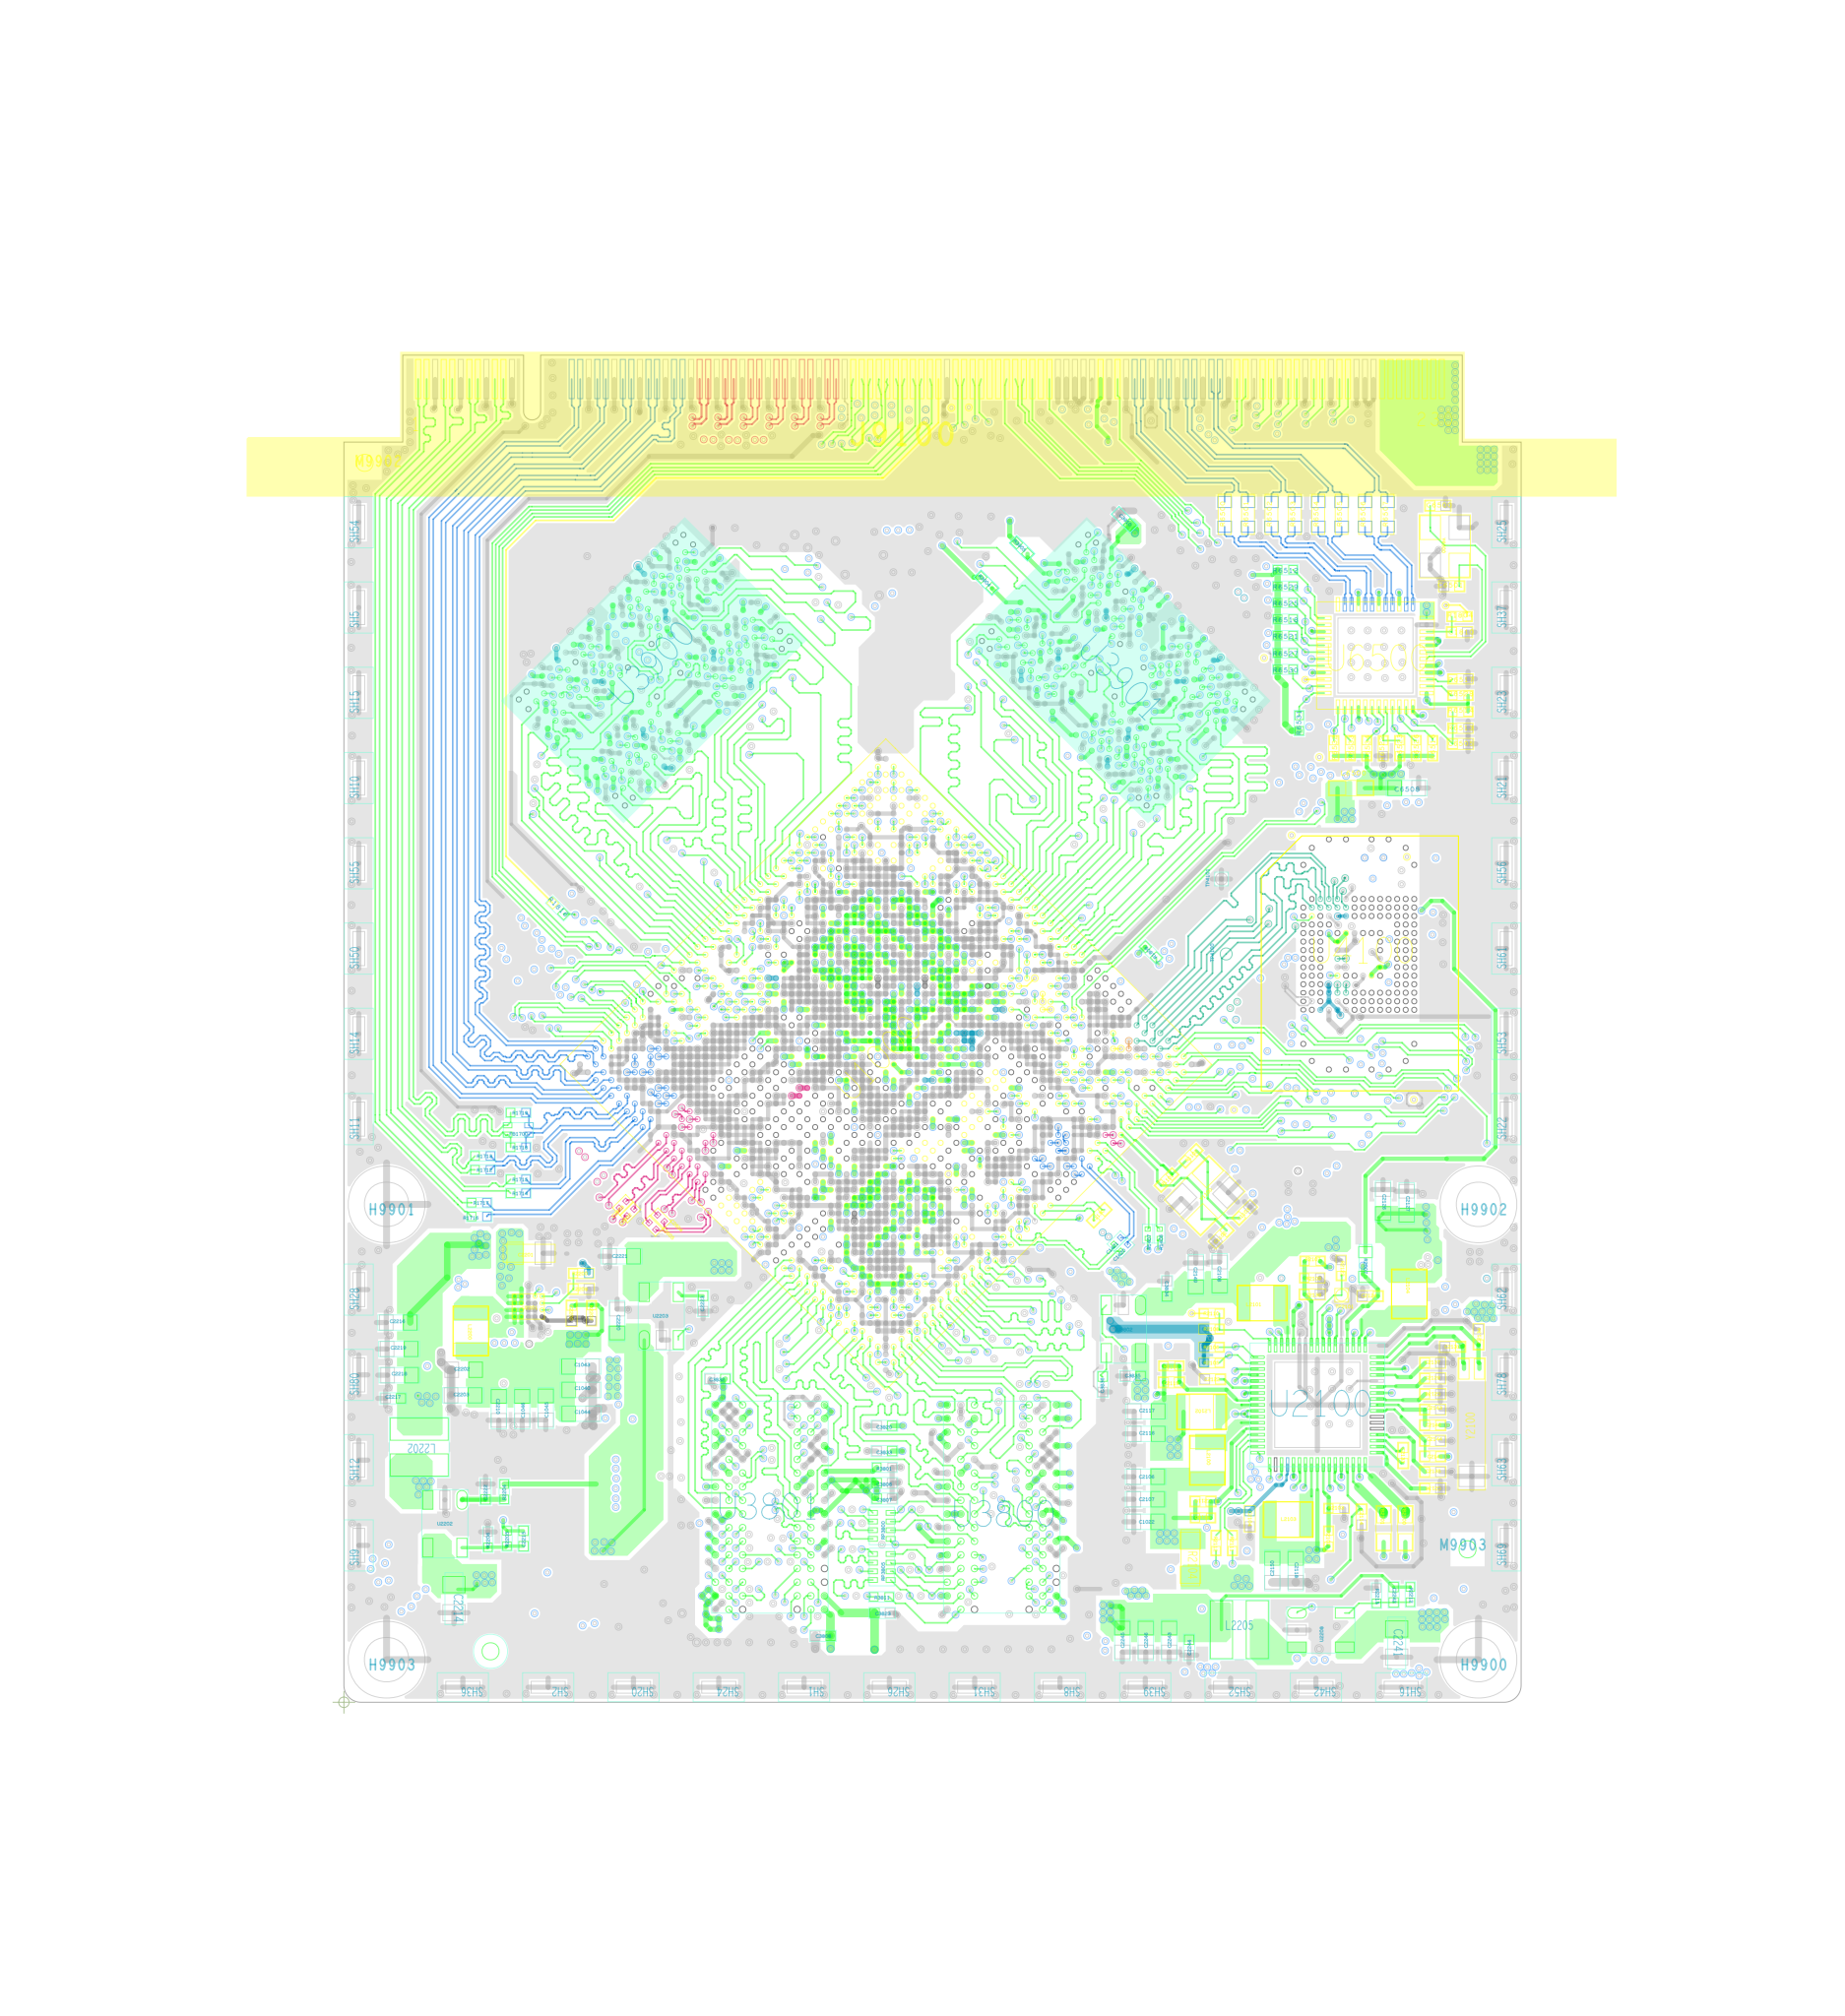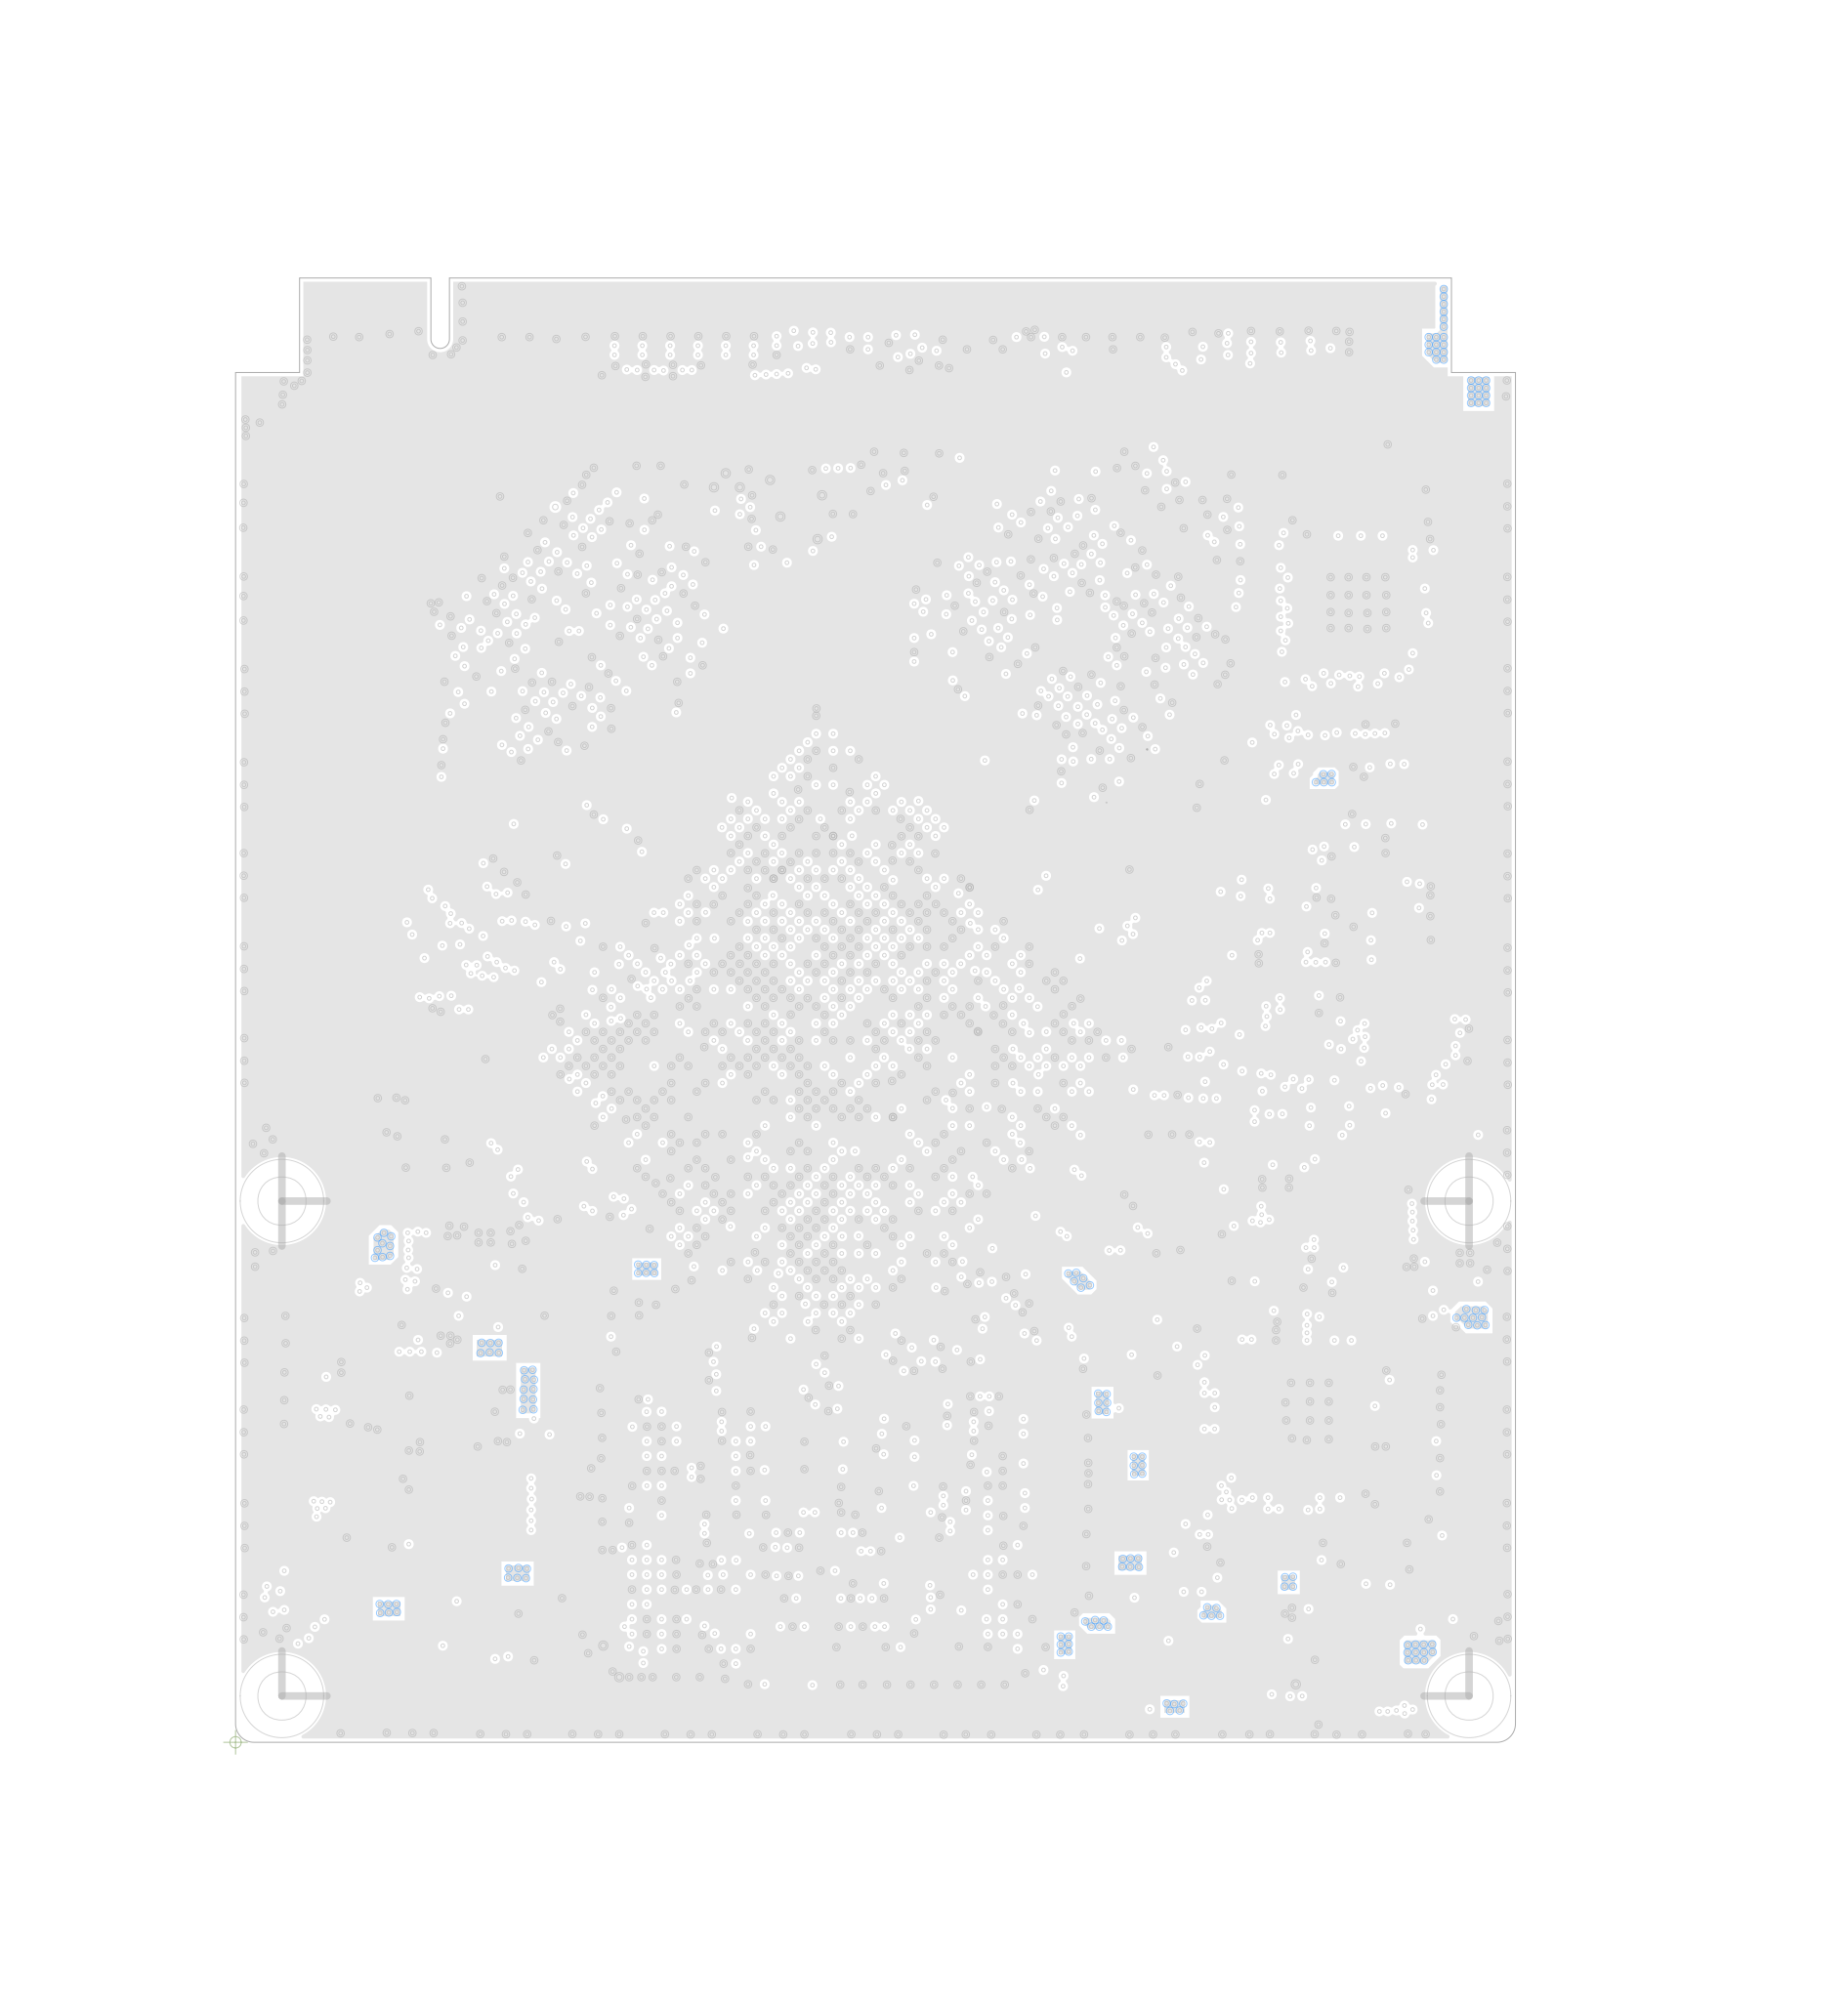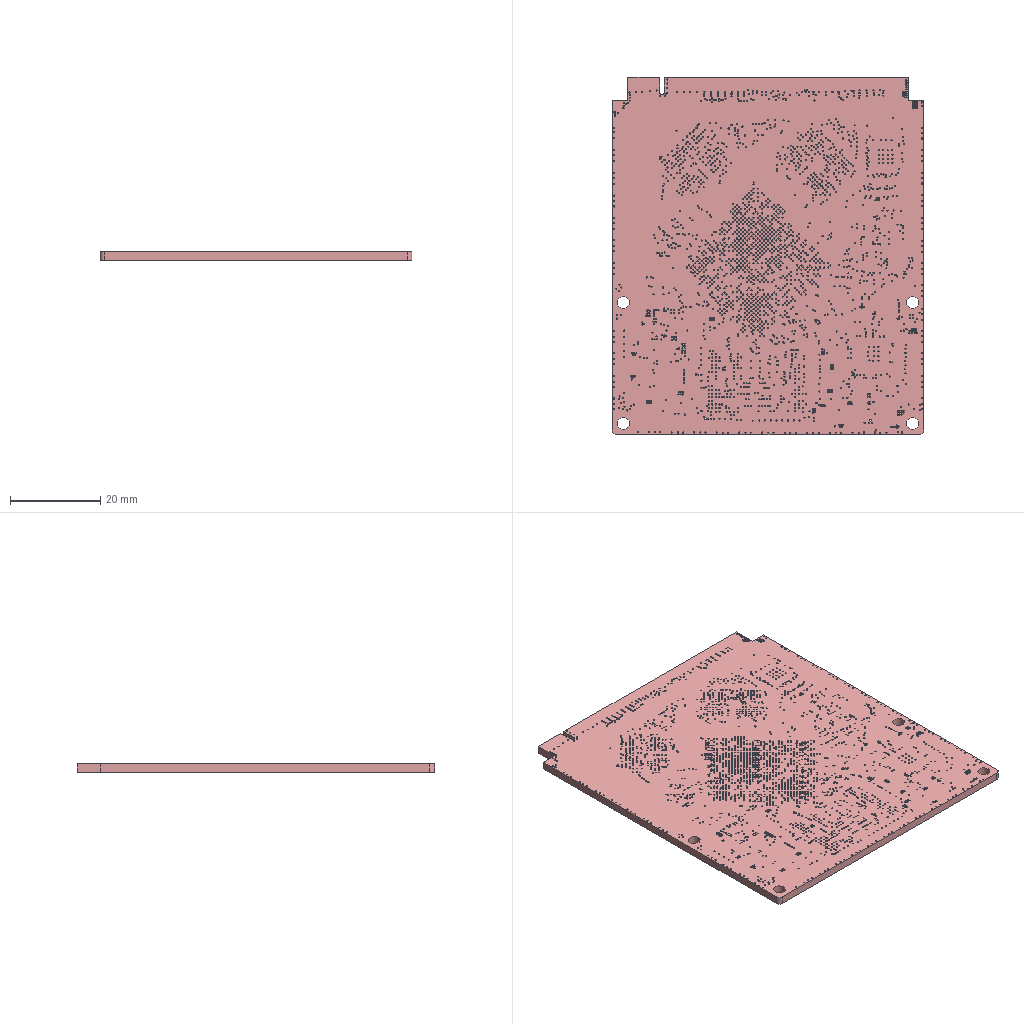Circuit board layout | Cadence Allegro | box 69 x 79 x 1.8 mm
Layer stack:
# Cadence Allegro layer stack of  (unit mm; from the constraint file cross-section; dielectric type: 0 not recorded (Allegro does not mark core vs prepreg), 3 surface material)
index,name,kind,layer,copper_thickness_mm,dielectric_type,dielectric_thickness_mm,dielectric_material,dielectric_constant
0,Top Surface,other,,,,,,
1,Dielectric1,dielectric,,,3,0.0249,FR-4,3.5
2,TOP,copper,TOP,0.0351,,,,
3,Dielectric2,dielectric,,,0,0.0749,FR-4,3.8
4,GND1,copper,GND1,0.017,,,,
5,Dielectric3,dielectric,,,0,0.365,FR-4,4.5
6,POWER1,copper,POWER1,0.017,,,,
7,Dielectric4,dielectric,,,0,0.1151,FR-4,4.5
8,POWER2,copper,POWER2,0.017,,,,
9,Dielectric5,dielectric,,,0,0.2649,FR-4,4.5
10,GND2,copper,GND2,0.017,,,,
11,Dielectric6,dielectric,,,0,0.1151,FR-4,4.5
12,S1,copper,S1,0.017,,,,
13,Dielectric7,dielectric,,,0,0.2032,FR-4,4.5
14,GND3,copper,GND3,0.0305,,,,
15,Dielectric8,dielectric,,,0,0.2032,FR-4,4.5
16,S2,copper,S2,0.0305,,,,
17,Dielectric9,dielectric,,,0,0.2032,FR-4,4.5
18,GND4,copper,GND4,0.017,,,,
19,Dielectric10,dielectric,,,0,0.0749,FR-4,3.8
20,BOTTOM,copper,BOTTOM,0.0351,,,,
21,Dielectric11,dielectric,,,3,0.0249,FR-4,3.5
22,Bottom Surface,other,,,,,,
# drill layer pairs: low layer,high layer
drill_pair,TOP,BOTTOM
Part placement, first 491 of 754 lines:
REFDES,COMP_VALUE,SYM_NAME,SYM_X,SYM_Y,SYM_ROTATE,SYM_MIRROR
C1000,22uF,C0603,1929.38,477.69,90.000,YES
C1001,22uF,C0603,1984.88,478.69,90.000,YES
C1002,1uF,C0402,1887.38,550.69,0.000,YES
C1003,100nF,C0201,1365.38,1521.69,45.000,YES
C1004,100nF,C0201,1318.38,1632.69,315.000,YES
C1005,100nF,C0201,1408.38,1542.69,135.000,YES
C1006,100nF,C0201,1305.38,1588.69,45.000,YES
C1007,1nF,C0201,1334.38,1539.69,135.000,YES
C1008,10uF,C0402,1370.38,1575.69,225.000,YES
C1009,10uF,C0402,1366.38,1657.69,45.000,YES
C1010,10uF,C0402,1209.38,1485.69,45.000,YES
C1011,22uF,C0603,2206.88,1161.69,270.000,YES
C1012,22uF,C0603,1558.38,1504.19,225.000,YES
C1013,22uF,C0603,2262.88,1162.69,270.000,YES
C1014,1uF,C0402,1488.88,1435.69,45.000,YES
C1015,100nF,C0201,1393.38,1713.69,225.000,YES
C1016,100nF,C0201,1450.38,1650.69,315.000,YES
C1017,100nF,C0201,1469.38,1679.69,225.000,YES
C1018,100nF,C0201,1431.38,1700.69,135.000,YES
C1019,100nF,C0201,1465.38,1593.69,135.000,YES
C1020,1nF,C0201,1413.38,1682.69,135.000,YES
C1021,10uF,C0402,1216.88,1587.69,45.000,YES
C1022,22uF,C0603,1850.38,416.69,180.000,NO
C1023,10uF,C0402,1282.38,1697.69,135.000,YES
C1024,1uF,C0402,1752.38,1630.69,45.000,YES
C1025,100nF,C0201,1222.38,1814.69,315.000,YES
C1026,100nF,C0201,1251.38,1781.41,45.000,YES
C1027,100nF,C0201,1305.38,1759.69,225.000,YES
C1028,100nF,C0201,1290.38,1776.69,225.000,YES
C1029,1nF,C0201,1252.38,1745.41,225.000,YES
C1030,22uF,C0603,2001.38,288.69,0.000,YES
C1031,10uF,C0402,1230.38,1452.19,45.000,YES
C1032,1uF,C0402,1286.38,1508.19,45.000,YES
C1033,100nF,C0201,1342.38,1724.41,315.000,YES
C1034,100nF,C0201,1325.38,1491.69,45.000,YES
C1035,100nF,C0201,1283.38,1604.69,225.000,YES
C1036,100nF,C0201,1256.38,1525.69,45.000,YES
C1037,1nF,C0201,1250.38,1564.69,45.000,YES
C1038,10uF,C0402,1265.38,1822.69,315.000,YES
C1039,22uF,C0603,829.38,1413.69,0.000,YES
C1040,22uF,C0603,546.38,721.19,0.000,NO
C1041,22uF,C0603,1150.38,1617.69,45.000,YES
C1042,22uF,C0603,1100.38,1678.69,45.000,YES
C1043,22uF,C0603,545.88,775.19,0.000,NO
C1044,22uF,C0603,546.38,666.19,0.000,NO
C1045,22uF,C0603,465.88,679.69,270.000,NO
C1046,22uF,C0603,411.38,678.69,270.000,NO
C1047,1uF,C0402,1210.88,1660.19,135.000,YES
C1048,100nF,C0201,1172.88,1704.69,315.000,YES
C1049,100nF,C0201,1158.38,1756.69,315.000,YES
C1050,100nF,C0201,1214.38,1751.69,225.000,YES
C1051,100nF,C0201,1217.38,1705.69,135.000,YES
C1052,100nF,C0201,1196.38,1769.69,225.000,YES
C1053,100nF,C0201,1177.38,1590.69,45.000,YES
C1054,1nF,C0201,1145.38,1667.69,45.000,YES
C1055,22uF,C0603,1576.38,1028.69,135.000,YES
C1056,100nF,C0201,1234.38,1032.69,135.000,YES
C1057,100nF,C0201,1260.38,1111.69,315.000,YES
C1058,100nF,C0201,1252.38,1050.69,135.000,YES
C1059,22uF,C0603,1027.25,1065.83,0.000,YES
C1060,100nF,C0201,1231.38,1223.69,315.000,YES
C1061,100nF,C0201,1153.38,1109.69,135.000,YES
C1062,100nF,C0201,1154.38,1148.69,315.000,YES
C1063,100nF,C0201,1173.38,1166.69,315.000,YES
C1064,100nF,C0201,1194.38,1186.69,315.000,YES
C1065,100nF,C0201,1225.38,1147.69,135.000,YES
C1066,100nF,C0201,1213.38,1205.69,315.000,YES
C1067,100nF,C0201,1240.38,1182.69,225.000,YES
C1068,4.7uF,C0402,1210.38,1116.69,135.000,YES
C1069,10uF,C0402,1648.38,1036.69,135.000,YES
C1070,100nF,C0201,1282.38,1161.69,315.000,YES
C1071,100nF,C0201,1264.38,1143.69,315.000,YES
C1072,100nF,C0201,1158.38,1236.69,225.000,YES
C1073,22uF,C0603,941.91,983.04,90.000,YES
C1080,100nF,C0201,1310.38,1016.69,45.000,YES
C1100,100nF,C0201,2141.38,828.69,270.000,YES
C1101,DNP,C0402,1985.38,1343.69,0.000,YES
C1102,18pF,C0402,2024.38,1076.69,225.000,NO
C1103,18pF,C0402,2078.38,1130.69,225.000,NO
C1104,100nF,C0201,1488.38,1548.69,225.000,YES
C1105,100nF,C0201,1466.38,1522.69,135.000,YES
C1106,100nF,C0201,1402.38,1474.41,315.000,YES
C1107,100nF,C0201,1506.38,1510.41,45.000,YES
C1108,100nF,C0201,1444.38,1506.69,135.000,YES
C1109,100nF,C0201,1269.38,1660.69,315.000,YES
C1110,100nF,C0201,1449.38,1554.69,225.000,YES
C1111,100nF,C0201,1430.38,1572.69,225.000,YES
C1112,100nF,C0402,1589.88,1438.69,45.000,YES
C1115,100nF,C0201,1282.38,1202.69,315.000,YES
C1116,100nF,C0201,1306.38,1228.41,225.000,YES
C1117,100nF,C0201,1341.38,1191.69,225.000,YES
C1118,100nF,C0201,1323.38,1208.69,225.000,YES
C1119,100nF,C0201,1078.38,1220.41,90.000,YES
C1120,100nF,C0201,1380.38,1170.41,225.000,YES
C1126,100nF,C0201,1158.38,1200.41,45.000,YES
C1130,100nF,C0402,1742.88,1124.69,225.000,NO
C1200,22uF,C0603,1548.38,1818.41,225.000,YES
C1201,10uF,C0402,1889.38,2511.41,225.000,YES
C1202,1uF,C0402,1076.33,1758.69,315.000,YES
C1203,100nF,C0201,1376.38,1790.69,225.000,YES
C1204,100nF,C0201,1393.38,1772.69,225.000,YES
C1205,100nF,C0201,1179.38,1788.69,225.000,YES
C1206,100nF,C0201,1198.38,1872.69,315.000,YES
C1207,100nF,C0201,1358.38,1808.69,225.000,YES
C1208,100nF,C0201,1116.38,1794.41,315.000,YES
C1209,1uF,C0402,1920.38,2110.41,45.000,YES
C1210,100nF,C0201,1136.38,1886.41,315.000,YES
C1211,1uF,C0402,982.38,1811.69,315.000,YES
C1212,100nF,C0201,1384.38,1892.41,225.000,YES
C1213,22uF,C0603,1241.38,2033.65,270.000,YES
C1214,10uF,C0402,1300.38,1885.41,225.000,YES
C1215,1uF,C0402,1336.38,1834.69,225.000,YES
C1216,100nF,C0201,1178.38,1852.69,315.000,YES
C1217,100nF,C0201,1413.38,1757.69,225.000,YES
C1218,100nF,C0201,1139.38,1738.69,135.000,YES
C1219,100nF,C0201,1160.38,1834.69,315.000,YES
C1220,100nF,C0201,1255.38,1906.41,225.000,YES
C1221,100nF,C0201,1098.38,1776.41,315.000,YES
C1222,1uF,C0402,2176.38,443.69,90.000,YES
C1223,100nF,C0201,1137.38,1821.41,315.000,YES
C1224,1uF,C0402,2140.38,443.69,90.000,YES
C1225,100nF,C0201,1395.38,1859.41,225.000,YES
C1226,4.7uF,C0402,1362.38,996.69,135.000,YES
C1227,1uF,C0402,1238.38,939.69,135.000,YES
C1228,100nF,C0201,1146.38,1032.69,45.000,YES
C1229,100nF,C0201,1176.38,1023.69,225.000,YES
C1230,100nF,C0201,1276.38,965.69,315.000,YES
C1231,100nF,C0201,1294.38,982.69,315.000,YES
C1232,100nF,C0201,1211.38,987.69,225.000,YES
C1233,100nF,C0201,1142.38,1064.69,45.000,YES
C1234,100nF,C0201,1178.38,968.69,135.000,YES
C1235,100nF,C0201,1194.38,1005.39,225.000,YES
C1300,100nF,C0201,1516.38,1578.69,135.000,YES
C1301,100nF,C0201,1544.38,1588.41,135.000,YES
C1400,100nF,C0201,1368.38,1414.41,135.000,YES
C1401,100nF,C0201,1389.88,1424.69,135.000,YES
C1402,100nF,C0201,1222.38,1539.69,315.000,YES
C1403,100nF,C0201,1235.88,1413.69,45.000,YES
C1404,100nF,C0201,1140.38,1482.69,45.000,YES
C1405,100nF,C0201,1284.38,1457.69,45.000,YES
C1406,100nF,C0201,1192.38,1519.69,225.000,YES
C1407,100nF,C0201,1320.38,1422.13,315.000,YES
C1416,100nF,C0201,1353.38,1098.69,135.000,YES
C1417,100nF,C0201,1398.38,1152.41,225.000,YES
C1418,100nF,C0201,1306.38,1066.69,45.000,YES
C1419,100nF,C0201,1282.38,1023.69,45.000,YES
C1420,100nF,C0201,1800.88,1048.91,45.000,NO
C1421,100nF,C0201,1784.88,1064.91,45.000,NO
C1422,100nF,C0201,1634.38,1116.41,180.000,YES
C1423,100nF,C0201,1634.38,1138.41,180.000,YES
C1424,100nF,C0201,1596.38,1316.41,180.000,YES
C1425,100nF,C0201,1596.38,1294.41,180.000,YES
C1426,100nF,C0201,1630.38,1198.41,180.000,YES
C1427,100nF,C0201,1630.38,1176.41,180.000,YES
C1428,100nF,C0201,1682.38,1076.41,180.000,YES
C1429,100nF,C0201,1682.38,1098.41,180.000,YES
C1430,100nF,C0201,1370.38,1471.69,315.000,YES
C1431,100nF,C0201,1422.38,1444.41,45.000,YES
C1433,100nF,C0201,1285.38,1411.69,135.000,YES
C1434,100nF,C0201,1195.26,1237.47,225.000,YES
C1500,100nF,C0201,1286.38,1372.69,45.000,YES
C1501,1nF,C0201,1402.38,1335.19,45.000,YES
C1502,100nF,C0402,1338.38,1300.69,45.000,YES
C1601,DNP,C0402,1864.70,1610.51,225.000,YES
C1602,100nF,C0201,1497.88,1626.69,315.000,YES
C1603,100nF,C0201,1479.38,1610.69,315.000,YES
C1604,100nF,C0201,1088.38,1098.41,315.000,YES
C1700,100nF,C0201,1069.38,1606.69,225.000,YES
C1701,100nF,C0201,1108.38,1545.69,225.000,YES
C1702,100nF,C0201,994.38,1588.69,45.000,YES
C1703,100nF,C0201,1074.38,1468.69,45.000,YES
C1704,100nF,C0201,1177.38,1537.69,225.000,YES
C1722,4.7uF,C0402,1133.92,1535.73,45.000,YES
C1723,4.7uF,C0402,1038.38,1504.69,315.000,YES
C1726,100nF,C0201,1089.38,1183.69,0.000,YES
C1727,100nF,C0201,1069.38,1155.69,0.000,YES
C1800,100nF,C0201,1384.38,1506.41,45.000,YES
C1801,100nF,C0201,1466.38,1454.41,45.000,YES
C1802,100nF,C0201,991.04,1682.05,225.000,YES
C1803,100nF,C0201,1054.38,1708.41,135.000,YES
C1804,100nF,C0201,1014.38,1662.41,225.000,YES
C1805,100nF,C0201,965.94,1644.04,315.000,YES
C1806,100nF,C0201,1494.38,1667.69,225.000,YES
C1807,100nF,C0201,1036.38,1690.41,135.000,YES
C1808,100nF,C0201,1547.38,1621.69,135.000,YES
C1810,DNP,C0402,2574.38,2470.69,0.000,NO
C2100,10uF,C0603,2218.38,583.69,270.000,YES
C2101,1uF,C0402,2296.38,567.69,270.000,YES
C2102,1uF,C0402,2104.38,443.69,90.000,YES
C2103,10uF,C0603,2143.38,656.69,0.000,YES
C2104,1uF,C0402,2090.38,423.69,270.000,NO
C2105,1uF,C0402,2138.38,567.69,270.000,YES
C2106,22uF,C0603,1850.38,520.69,180.000,NO
C2107,10uF,C0603,1850.38,468.69,180.000,NO
C2108,22uF,C0603,2020.88,988.69,90.000,NO
C2109,1uF,C0402,2262.38,567.69,270.000,YES
C2110,100pF,C0402,1982.38,463.69,0.000,NO
C2111,10uF,C0603,2197.38,790.69,90.000,YES
C2112,1uF,C0402,2174.38,567.69,270.000,YES
C2113,1uF,C0402,2350.38,492.69,180.000,YES
C2114,1uF,C0402,2348.38,427.69,270.000,NO
C2115,1uF,C0402,2130.38,774.69,180.000,YES
C2116,22uF,C0603,1851.38,619.69,180.000,NO
C2117,10uF,C0603,1851.38,671.69,180.000,NO
C2118,22uF,C0603,2196.38,304.69,270.000,NO
C2119,100pF,C0402,1909.38,738.69,180.000,NO
C2120,1uF,C0402,2130.38,702.69,180.000,YES
C2121,1uF,C0402,2130.38,738.69,180.000,YES
C2122,1uF,C0402,2004.38,745.69,180.000,NO
C2123,1uF,C0402,2272.38,809.69,90.000,YES
C2124,1uF,C0402,2368.38,937.69,180.000,NO
C2125,1uF,C0402,2308.38,809.69,90.000,YES
C2126,22uF,C0603,2397.88,1156.19,90.000,NO
C2127,22uF,C0603,2452.38,1152.19,90.000,NO
C2128,10uF,C0603,2354.38,793.69,90.000,YES
C2129,1uF,C0402,2512.38,747.69,180.000,NO
C2130,1uF,C0402,2365.38,675.69,180.000,YES
C2131,22pF,C0402,2558.38,820.69,0.000,NO
C2132,10uF,C0603,2340.38,583.69,270.000,YES
C2133,2.2uF,C0402,2444.38,569.69,90.000,NO
C2134,22pF,C0402,2618.38,843.69,270.000,NO
C2135,1uF,C0402,2512.38,531.69,180.000,NO
C2136,2.2uF,C0402,2512.38,493.69,180.000,NO
C2137,1uF,C0402,2512.38,783.69,180.000,NO
C2138,1uF,C0402,2512.38,711.69,180.000,NO
C2139,100nF,C0402,2234.38,941.69,0.000,NO
C2140,100nF,C0402,2512.38,639.69,180.000,NO
C2141,100nF,C0402,2512.38,567.69,180.000,NO
C2142,100nF,C0402,2367.38,909.69,270.000,YES
C2143,27pF,C0402,2512.38,675.69,0.000,NO
C2144,27pF,C0402,2512.38,603.69,0.000,NO
C2145,100nF,C0402,2108.38,836.69,90.000,YES
C2146,1uF,C0402,1994.38,918.69,90.000,YES
C2149,10uF,C0603,1965.88,986.69,90.000,NO
C2150,10uF,C0603,2142.38,304.69,270.000,NO
C2200,100nF,C0402,525.38,898.19,90.000,NO
C2201,10uF,C0805,427.38,1036.69,0.000,NO
C2202,22uF,C0603,276.38,767.69,180.000,NO
C2203,22uF,C0603,274.88,708.69,180.000,NO
C2204,100nF,C0402,2310.88,1178.69,90.000,YES
C2205,10uF,C0805,2508.38,786.69,90.000,YES
C2206,22uF,C0603,2151.88,1159.69,270.000,YES
C2207,22uF,C0603,2429.38,1174.69,180.000,YES
C2208,100nF,C0402,547.38,954.19,0.000,NO
C2209,100nF,C0402,2574.39,960.69,270.000,YES
C2210,22uF,C0603,357.38,678.69,270.000,NO
C2211,22uF,C0603,542.88,768.69,90.000,YES
C2212,22uF,C0603,2320.38,1037.69,90.000,YES
C2213,22uF,C0603,2218.88,1033.69,90.000,YES
C2214,10uF,C0805,253.88,239.19,270.000,NO
C2215,22pF,C0402,414.38,378.19,270.000,NO
C2216,22uF,C0603,125.38,876.69,180.000,NO
C2217,100nF,C0402,113.88,701.69,180.000,NO
C2218,22uF,C0603,128.38,755.19,180.000,NO
C2219,10uF,C0603,127.38,815.69,180.000,NO
C2220,4.7uF,C0603,630.38,880.19,90.000,NO
C2221,4.7uF,C0603,640.88,1029.69,180.000,NO
C2222,100nF,C0402,326.88,486.19,90.000,NO
C2223,100nF,C0402,828.88,920.69,270.000,NO
C2224,4.7uF,C0603,185.38,632.69,0.000,YES
C2225,4.7uF,C0603,237.38,919.69,0.000,YES
C2226,10uF,C0805,427.88,1040.19,180.000,YES
C2227,100nF,C0402,139.38,869.69,270.000,YES
C2228,47uF,C0805,724.38,876.69,180.000,YES
C2229,47uF,C0805,724.38,796.69,180.000,YES
C2230,47uF,C0805,724.38,958.69,180.000,YES
C2231,47uF,C0805,724.38,716.69,180.000,YES
C2232,4.7uF,C0603,1936.88,685.69,0.000,YES
C2233,22pF,C0402,1791.88,912.19,90.000,YES
C2234,4.7uF,C0603,1925.88,966.19,270.000,YES
C2235,10uF,C0805,2406.38,242.69,270.000,YES
C2236,100pF,C0402,2423.38,129.69,270.000,YES
C2237,22uF,C0603,1797.38,142.69,90.000,YES
C2238,100nF,C0402,1957.38,130.69,90.000,YES
C2239,22uF,C0603,1851.38,142.69,90.000,YES
C2240,10uF,C0603,1906.38,143.69,90.000,YES
C2241,10uF,C0805,2429.38,136.69,270.000,NO
C2242,22pF,C0402,2422.38,248.19,270.000,NO
C2243,22uF,C0603,1904.38,143.69,270.000,NO
C2244,100nF,C0402,1950.38,126.69,270.000,NO
C2245,22uF,C0603,1796.38,143.69,270.000,NO
C2246,10uF,C0603,1850.38,143.69,270.000,NO
C2250,10uF,C0805,172.88,550.69,0.000,YES
C2251,22pF,C0402,438.88,664.19,0.000,YES
C2252,22uF,C0603,680.38,501.69,180.000,YES
C2253,100nF,C0402,680.38,613.69,180.000,YES
C2254,22uF,C0603,680.38,561.69,180.000,YES
C2255,10uF,C0603,680.38,445.69,180.000,YES
C2260,100nF,C0402,439.38,787.69,180.000,YES
C2310,1uF,C0402,2365.38,713.69,0.000,YES
C2600,100nF,C0201,547.14,1183.38,180.000,YES
C2601,100nF,C0201,546.43,1209.54,180.000,YES
C2602,100nF,C0201,661.38,1130.69,225.000,NO
C2603,100nF,C0201,643.38,1148.69,225.000,NO
C2604,100nF,C0201,731.49,1117.50,315.000,NO
C2605,100nF,C0201,711.99,1099.50,315.000,NO
C2606,220pF,C0402,2332.38,1925.69,0.000,YES
C2607,220pF,C0402,2412.38,1925.69,180.000,YES
C2608,1uF,C0402,2498.38,1798.69,180.000,YES
C2609,100nF,C0402,2499.38,1926.69,0.000,YES
C3800,100pF,C0201,974.88,490.61,180.000,YES
C3801,100nF,C0402,814.02,284.06,270.000,YES
C3802,100nF,C0402,793.04,224.96,0.000,YES
C3803,100nF,C0402,1702.38,183.70,180.000,YES
C3804,100nF,C0402,1445.72,439.04,180.000,YES
C3805,100nF,C0402,1234.28,514.61,180.000,YES
C3806,100nF,C0402,1247.33,506.21,0.000,NO
C3807,100nF,C0402,1247.33,470.21,0.000,NO
C3808,100nF,C0402,1105.38,153.41,180.000,NO
C3809,100nF,C0402,1315.06,514.02,0.000,YES
C3810,100nF,C0402,1545.74,840.59,135.000,YES
C3811,100nF,C0402,1271.85,412.06,0.000,YES
C3812,100nF,C0402,1109.25,540.15,0.000,YES
C3813,100nF,C0402,1019.41,516.88,0.000,YES
C3814,100nF,C0402,1639.44,495.39,0.000,YES
C3815,100nF,C0402,794.21,437.06,0.000,YES
C3816,100nF,C0402,830.13,608.20,0.000,YES
C3817,100nF,C0402,794.21,496.44,0.000,YES
C3818,100nF,C0402,814.03,364.71,270.000,YES
C3819,1nF,C0402,1342.65,337.59,0.000,YES
C3820,100nF,C0402,1247.33,638.41,180.000,NO
C3821,100nF,C0402,830.13,648.92,0.000,YES
C3822,100nF,C0402,1702.38,220.70,180.000,YES
C3823,100nF,C0402,1242.28,206.21,0.000,NO
C3824,22uF,C0603,810.38,178.41,0.000,YES
C3825,22uF,C0603,844.37,764.08,0.000,YES
C3826,22uF,C0603,1642.37,680.77,270.000,YES
C3827,100nF,C0402,1109.39,595.09,0.000,YES
C3828,100nF,C0402,1123.12,696.13,315.000,YES
C3829,100nF,C0402,830.13,699.66,0.000,YES
C3830,100nF,C0402,1669.88,377.12,0.000,YES
C3831,100nF,C0402,1248.89,606.99,315.000,YES
C3832,100nF,C0402,862.33,746.70,180.000,NO
C3833,100nF,C0402,1247.33,580.12,180.000,NO
C3834,1uF,C0402,1899.38,954.69,90.000,NO
C3835,4.7uF,C0402,1820.88,753.19,180.000,NO
C3836,100nF,C0402,1750.88,734.19,270.000,NO
C3900,22uF,C0603,438.39,2284.70,90.000,YES
C3901,1uF,C0402,1786.37,2695.43,0.000,YES
C3902,100nF,C0402,675.82,2065.57,45.000,YES
C3903,100nF,C0402,862.56,2450.80,0.000,YES
C3904,100nF,C0402,575.37,2242.03,225.000,YES
C3905,100nF,C0402,891.81,2572.81,225.000,YES
C3906,100nF,C0402,652.07,2093.82,225.000,YES
C3907,100nF,C0402,700.38,2190.55,135.000,YES
C3908,22uF,C0603,1780.99,2742.80,0.000,YES
C3909,1uF,C0402,1922.70,2232.04,135.000,YES
C3910,100nF,C0402,1801.35,2730.42,135.000,NO
C3911,100nF,C0402,1993.02,2239.24,135.000,YES
C3912,100nF,C0402,2083.66,2384.32,135.000,YES
C3913,100nF,C0402,1965.97,2168.11,135.000,YES
C3914,100nF,C0402,1674.14,2534.13,225.000,YES
C3915,100nF,C0402,1897.16,2135.68,225.000,YES
C3916,10uF,C0603,604.38,2639.55,315.000,YES
C3917,100nF,C0402,764.35,2429.13,45.000,YES
C3918,100nF,C0402,460.38,2418.69,45.000,YES
C3919,100nF,C0402,707.45,2319.58,225.000,YES
C3920,10uF,C0603,1878.41,2646.99,225.000,YES
C3921,100nF,C0402,2027.38,2444.70,315.000,YES
C3922,100nF,C0402,1725.38,2355.55,135.000,YES
C3923,100nF,C0402,1808.38,2241.55,315.000,YES
C3924,10uF,C0603,1828.67,2298.27,315.000,YES
C3925,1uF,C0402,499.38,2248.18,225.000,YES
C3926,100nF,C0402,543.63,2471.72,45.000,YES
C3927,100nF,C0402,612.37,2535.20,225.000,YES
C3928,100nF,C0402,792.62,2486.81,135.000,YES
C3929,100nF,C0402,634.23,2299.68,45.000,YES
C3930,100nF,C0402,589.16,2076.10,135.000,YES
C3931,100nF,C0402,795.38,2305.55,135.000,YES
C3932,10uF,C0603,1043.41,2643.91,270.000,YES
C3933,1uF,C0402,1654.28,2630.89,180.000,YES
C3934,100nF,C0402,1700.38,2475.55,315.000,YES
C3935,100nF,C0402,1711.38,2293.55,180.000,YES
C3936,100nF,C0402,1584.20,2314.12,90.000,YES
C3937,100nF,C0402,2059.52,2260.21,225.000,YES
C3938,100nF,C0402,1858.66,2563.68,135.000,YES
C3939,100nF,C0402,1965.54,2497.71,135.000,YES
C3940,100nF,C0402,933.38,2289.34,90.000,YES
C3941,100nF,C0402,1503.01,2498.76,45.000,YES
C3942,100nF,C0402,836.70,2618.86,45.000,YES
C3943,100nF,C0402,826.84,2199.77,45.000,YES
C4100,2.2uF,C0402,2192.88,1849.69,90.000,YES
C4101,4.7uF,C0402,2317.88,1559.69,90.000,YES
C4102,100nF,C0402,2280.88,1559.19,90.000,YES
C4103,100nF,C0402,2260.88,1831.19,270.000,YES
C4104,4.7uF,C0402,2480.38,1648.69,180.000,YES
C4105,100nF,C0402,2480.38,1694.69,180.000,YES
C6500,12pF,C0402,2524.38,2762.69,0.000,NO
C6501,12pF,C0402,2556.38,2576.69,180.000,NO
C6504,100pF,C0402,2450.38,2318.69,270.000,YES
C6505,100pF,C0402,2576.38,2212.69,0.000,NO
C6506,100nF,C0402,2486.38,2452.69,0.000,YES
C6507,100nF,C0402,2272.38,2534.69,180.000,YES
C6508,10uF,C0603,2452.38,2110.69,0.000,NO
C6509,100nF,C0402,2396.38,2524.69,90.000,YES
C6510,100nF,C0402,2272.38,2496.69,180.000,YES
C6511,100nF,C0402,2276.38,2339.69,180.000,YES
C6512,10nF,C0402,2374.38,2318.69,270.000,YES
C6513,10uF,C0603,2254.38,2716.69,0.000,YES
C6514,100nF,C0402,2266.38,2666.69,0.000,YES
C6515,100nF,C0402,2494.88,2245.69,90.000,YES
C6516,100nF,C0402,2336.38,2318.69,270.000,YES
C6517,100nF,C0402,2358.38,2524.69,90.000,YES
C6518,100nF,C0402,2434.38,2524.69,90.000,YES
C6519,100nF,C0402,2486.38,2378.69,0.000,YES
C6520,DNP,C0402,2276.38,2379.69,180.000,YES
C6521,10uF,C0603,2240.38,2286.69,0.000,YES
C6522,100nF,C0402,2486.38,2414.69,0.000,YES
C9103,1uF,C0402,2511.38,603.69,180.000,YES
C9600,100nF,C0402,2481.38,1738.69,180.000,YES
C9601,1uF,C0402,2191.88,1680.69,90.000,YES
C9602,100nF,C0402,2243.88,1557.19,90.000,YES
D2000,B5819WS,SOD_323,2597.88,781.19,90.000,YES
D2100,BAT54C,SOT_23,2045.38,1072.69,180.000,YES
D2600,BZT52C3V0,SOD_123,2506.38,2057.69,90.000,YES
FB1700,90R-100M,RP2_0504,402.38,1321.41,180.000,NO
FB2100,180R-100M,L0603,2449.38,401.69,270.000,NO
FB2101,180R-100M,L0603,2399.38,401.69,270.000,NO
H9900,SHIELD,HOLE_4P5TH2P6,2618.11,98.42,0.000,NO
H9901,SHIELD,HOLE_4P5TH2P6,98.43,1149.60,0.000,NO
H9902,SHIELD,HOLE_4P5TH2P6,2618.11,1149.60,0.000,NO
H9903,SHIELD,HOLE_4P5TH2P6,98.43,98.42,0.000,NO
J9100,AS0B326-S43N-7F,MXM_230P_0P5,1358.06,3110.23,0.000,NO
L2100,470nH,IND_252010,1992.38,558.19,270.000,NO
L2101,470nH,IND_252010,2118.38,921.69,180.000,NO
L2102,470nH,IND_252010,1978.88,670.69,180.000,NO
L2103,470nH,IND_252010,2178.38,421.69,180.000,NO
L2104,470nH,IND_252010,2458.38,942.19,270.000,NO
L2200,0.24uH,IND_252012,292.88,856.69,270.000,NO
L2201,0.24uH,IND_252012,2425.88,1085.69,0.000,YES
L2202,3.3uH,IND_303015,173.88,589.19,180.000,NO
L2203,0.24uH,IND_252012,577.38,951.69,180.000,YES
L2204,3.3uH,IND_303015,2068.38,166.69,270.000,YES
L2205,3.3uH,IND_303015,2066.38,167.69,270.000,NO
L2206,3.3uH,IND_303015,528.38,520.69,90.000,YES
L6500,180R-100M,L0603,2324.38,2110.69,0.000,NO
L6501,2.2uH,IND_303015,2408.38,2668.69,270.000,YES
M9900,MARK,MARK_C0100S0150M_S,51.38,2858.69,0.000,YES
M9901,MARK,MARK_C0100S0150M_S,2522.38,306.69,0.000,YES
M9902,MARK,MARK_C0100S0150M_S,47.88,2861.69,0.000,NO
M9903,MARK,MARK_C0100S0150M_S,2592.88,353.19,0.000,NO
Q2100,WNM2021,SOT_323,2109.38,938.69,180.000,YES
Q8202,WNM2021,SOT_323,288.38,1630.69,0.000,YES
Q8203,WNM2021,SOT_323,282.88,1794.69,0.000,YES
R1000,100R,R0201,1330.38,1056.69,225.000,YES
R1100,0R,R0402,2066.38,1344.20,180.000,YES
R1101,1M,R0402,1898.39,1205.68,45.000,NO
R1102,22R,R0402,1954.37,1261.70,225.000,NO
R1103,100R,R0402,2150.89,1680.69,90.000,YES
R1105,0R,R0402,1889.06,1363.66,180.000,YES
R1106,2.2K,R0402,2138.38,1538.70,180.000,YES
R1107,2.2K,R0402,2003.87,1541.20,225.000,YES
R1120,2.2K,R0402,2448.38,1433.69,180.000,YES
R1121,2.2K,R0402,2448.38,1471.69,180.000,YES
R1122,100K,R0402,1390.38,1246.41,45.000,YES
R1123,0R,R0402,1364.38,1273.69,225.000,YES
R1124,0R,R0402,1957.21,1415.25,270.000,YES
R1125,0R,R0402,1995.06,1415.07,270.000,YES
R1126,0R,R0402,1483.38,1302.41,225.000,YES
R1130,2.2K,R0402,1462.38,1214.41,225.000,YES
R1131,2.2K,R0402,1514.38,1266.41,45.000,YES
R1140,100R,R0402,1080.38,1318.41,0.000,YES
R1141,100R,R0402,1040.38,1264.41,0.000,YES
R1200,0R,R0402,1189.38,1916.41,45.000,YES
R1201,0R,R0402,1350.28,1940.48,180.000,YES
R1202,0R,R0402,2250.38,443.69,90.000,YES
R1203,0R,R0402,2212.38,443.69,90.000,YES
R1204,240R,R0402,1058.38,1822.41,45.000,YES
R1205,240R,R0402,1423.38,1828.41,225.000,YES
R1207,240R,R0402,1390.38,1070.41,225.000,YES
R1300,10K,R0201,1582.66,1597.19,225.000,YES
R1301,22R,R0402,1983.85,1578.21,225.000,YES
R1400,133R,R0402,1849.38,1247.69,0.000,YES
R1401,133R,R0402,1849.38,1207.19,180.000,YES
R1402,499R,R0402,1114.38,1408.69,225.000,YES
R1403,499R,R0402,1154.38,1372.69,45.000,YES
R1406,2.2R,R0201,1882.45,1081.60,90.000,NO
R1407,2.2R,R0201,1854.82,1081.77,90.000,NO
R1408,1R,R0201,1298.38,1108.41,315.000,YES
R1409,1R,R0201,1125.38,1081.69,225.000,YES
R1410,47K,R0402,1492.38,1172.41,225.000,YES
R1418,2K,R0402,1434.38,1110.41,135.000,YES
R1422,1R,R0201,1338.38,1456.41,315.000,YES
R1423,1R,R0201,1440.88,1411.69,135.000,YES
R1424,1R,R0201,1368.38,1130.41,315.000,YES
R1425,1R,R0201,1324.38,1138.41,315.000,YES
R1500,10K,R0402,1427.88,1378.69,135.000,YES
R1501,100K,R0402,1356.38,1366.41,315.000,YES
R1502,100K,R0402,1457.38,1328.41,225.000,YES
R1601,22R,R0402,1807.09,1556.15,225.000,YES
Pad and via stacks, first 104 of 108 lines:
# Allegro (Cadence) via spans and padstacks; design units: ("mils" 2 100)
# via spans: padstack,start_layer,end_layer,net_example,count
0503,ETCH/TOP,ETCH/BOTTOM,VCC_1V8_S3,11
0402,ETCH/TOP,ETCH/BOTTOM,GND,2653
# Allegro padstack definitions: name,start_layer,end_layer,drill,plating,holeType,type
S_S0R55,"ETCH/TOP","ETCH/TOP",0.0,"PLATED","none","smd"
S_R0R80X0R90,"ETCH/TOP","ETCH/TOP",0.0,"PLATED","none","smd"
S_S0R50,"ETCH/TOP","ETCH/TOP",0.0,"PLATED","none","smd"
S_C0R30,"ETCH/TOP","ETCH/TOP",0.0,"NON_PLATED","none","smd"
S_R1R40X1R20,"ETCH/TOP","ETCH/TOP",0.0,"NON_PLATED","none","smd"
S_R0R965X0R80,"ETCH/TOP","ETCH/TOP",0.0,"NON_PLATED","none","smd"
S_R0R65X0R80,"ETCH/TOP","ETCH/TOP",0.0,"NON_PLATED","none","smd"
S_R0R95X1R30,"ETCH/TOP","ETCH/TOP",0.0,"PLATED","none","smd"
S_R0R25X0R30,"ETCH/TOP","ETCH/TOP",0.0,"NON_PLATED","none","smd"
SHAPEESD0402_R,"ETCH/TOP","ETCH/TOP",0.0,"PLATED","none","smd"
SHAPEESD0402_L,"ETCH/TOP","ETCH/TOP",0.0,"PLATED","none","smd"
S_R0R80X0R60,"ETCH/TOP","ETCH/TOP",0.0,"NON_PLATED","none","smd"
S_R0R80X1R10,"ETCH/TOP","ETCH/TOP",0.0,"NON_PLATED","none","smd"
S_R0R20X0R68,"ETCH/TOP","ETCH/TOP",0.0,"NON_PLATED","none","smd"
S_R0R40X0R75,"ETCH/TOP","ETCH/TOP",0.0,"NON_PLATED","none","smd"
S_R1R50X4R00,"ETCH/TOP","ETCH/TOP",0.0,"NON_PLATED","none","smd"
S_R0R70X2R00,"ETCH/TOP","ETCH/TOP",0.0,"NON_PLATED","none","smd"
S_R1R00X1R20,"ETCH/TOP","ETCH/TOP",0.0,"NON_PLATED","none","smd"
S_R3R40X1R30,"ETCH/TOP","ETCH/TOP",0.0,"NON_PLATED","none","smd"
S_C0R50,"ETCH/TOP","ETCH/TOP",0.0,"NON_PLATED","none","smd"
S_R0R279X0R533,"ETCH/TOP","ETCH/TOP",0.0,"NON_PLATED","none","smd"
S_C0R70,"ETCH/TOP","ETCH/TOP",0.0,"NON_PLATED","none","smd"
S_R0R70X1R00,"ETCH/TOP","ETCH/TOP",0.0,"NON_PLATED","none","smd"
S_O0R70X1R00,"ETCH/TOP","ETCH/TOP",0.0,"NON_PLATED","none","smd"
S_R0R50X0R30,"ETCH/TOP","ETCH/TOP",0.0,"NON_PLATED","none","smd"
S_S5R00,"ETCH/TOP","ETCH/TOP",0.0,"NON_PLATED","none","smd"
S_R0R15X0R80,"ETCH/TOP","ETCH/TOP",0.0,"NON_PLATED","none","smd"
S_R0R80X0R15,"ETCH/TOP","ETCH/TOP",0.0,"NON_PLATED","none","smd"
S_O0R80X0R15,"ETCH/TOP","ETCH/TOP",0.0,"NON_PLATED","none","smd"
S_R1R10X0R60,"ETCH/TOP","ETCH/TOP",0.0,"NON_PLATED","none","smd"
S_O1R10X0R60,"ETCH/TOP","ETCH/TOP",0.0,"NON_PLATED","none","smd"
S_R1R20X1R50,"ETCH/TOP","ETCH/TOP",0.0,"NON_PLATED","none","smd"
S_R1R20X0R60,"ETCH/TOP","ETCH/TOP",0.0,"NON_PLATED","none","smd"
S_C0R24,"ETCH/TOP","ETCH/TOP",0.0,"NON_PLATED","none","smd"
S_C0R38,"ETCH/TOP","ETCH/TOP",0.0,"NON_PLATED","none","smd"
S_R0R70X0R90,"ETCH/TOP","ETCH/TOP",0.0,"NON_PLATED","none","smd"
S_R0R30X2R60,"ETCH/TOP","ETCH/TOP",0.0,"NON_PLATED","none","smd"
S_R0R25X0R70,"ETCH/TOP","ETCH/TOP",0.0,"NON_PLATED","none","smd"
S_R0R70X0R25,"ETCH/TOP","ETCH/TOP",0.0,"PLATED","none","smd"
S_R1R50X0R25,"ETCH/TOP","ETCH/TOP",0.0,"NON_PLATED","none","smd"
REC1P1X2P6NOSP,"ETCH/TOP","ETCH/TOP",0.0,"PLATED","none","smd"
REC1P7X5P7,"ETCH/TOP","ETCH/TOP",0.0,"PLATED","none","smd"
REC0P8X1P5,"ETCH/TOP","ETCH/TOP",0.0,"NON_PLATED","none","smd"
REC1P8X3P6,"ETCH/TOP","ETCH/TOP",0.0,"NON_PLATED","none","smd"
REC1X2P9,"ETCH/TOP","ETCH/TOP",0.0,"NON_PLATED","none","smd"
S_C0R30_CUT,"ETCH/TOP","ETCH/TOP",0.0,"NON_PLATED","none","smd"
CIR1SM2,"ETCH/TOP","ETCH/TOP",0.0,"NON_PLATED","none","smd"
REC0P4X1P35,"ETCH/TOP","ETCH/TOP",0.0,"NON_PLATED","none","smd"
REC2P75X3P3SP3P5X3,"ETCH/TOP","ETCH/TOP",0.0,"NON_PLATED","none","smd"
REC0P5X1,"ETCH/TOP","ETCH/TOP",0.0,"PLATED","none","smd"
CIR1NOSP,"ETCH/TOP","ETCH/TOP",0.0,"NON_PLATED","none","smd"
SMD83_38,"ETCH/TOP","ETCH/TOP",0.0,"NON_PLATED","none","smd"
SMD28X9,"ETCH/TOP","ETCH/TOP",0.0,"PLATED","none","smd"
SMD210X209,"ETCH/TOP","ETCH/TOP",0.0,"PLATED","none","smd"
R1_2X1_1,"ETCH/TOP","ETCH/TOP",0.0,"PLATED","none","smd"
R1D80X1D90,"ETCH/TOP","ETCH/TOP",0.0,"PLATED","none","smd"
S1D90,"ETCH/TOP","ETCH/TOP",0.0,"PLATED","none","smd"
R1D00X1D60,"ETCH/TOP","ETCH/TOP",0.0,"PLATED","none","smd"
R1D60X2D10,"ETCH/TOP","ETCH/TOP",0.0,"PLATED","none","smd"
R0D40X1D40,"ETCH/TOP","ETCH/TOP",0.0,"NON_PLATED","none","smd"
SMD20_50,"ETCH/TOP","ETCH/TOP",0.0,"NON_PLATED","none","smd"
SMD80_93,"ETCH/TOP","ETCH/TOP",0.0,"PLATED","none","smd"
REC1X2P8,"ETCH/TOP","ETCH/TOP",0.0,"PLATED","none","smd"
REC0P6X1P7,"ETCH/TOP","ETCH/TOP",0.0,"NON_PLATED","none","smd"
M0100C0150SM,"ETCH/TOP","ETCH/TOP",0.0,"PLATED","none","smd"
S_S1R00,"ETCH/TOP","ETCH/TOP",0.0,"NON_PLATED","none","smd"
R0_3X2_3_B,"ETCH/BOTTOM","ETCH/BOTTOM",0.0,"PLATED","none","smd"
R0_3X2_3,"ETCH/TOP","ETCH/TOP",0.0,"PLATED","none","smd"
S_S1R45,"ETCH/TOP","ETCH/TOP",0.0,"NON_PLATED","none","smd"
S_R0R30X0R60,"ETCH/TOP","ETCH/TOP",0.0,"NON_PLATED","none","smd"
S_R0R60X0R30,"ETCH/TOP","ETCH/TOP",0.0,"NON_PLATED","none","smd"
S_S4R40,"ETCH/TOP","ETCH/TOP",0.0,"NON_PLATED","none","smd"
S_R0R80X0R20,"ETCH/TOP","ETCH/TOP",0.0,"NON_PLATED","none","smd"
S_R0R20X0R80,"ETCH/TOP","ETCH/TOP",0.0,"NON_PLATED","none","smd"
S_O0R20X0R80,"ETCH/TOP","ETCH/TOP",0.0,"NON_PLATED","none","smd"
2P0X0P7_MM_SMD,"ETCH/TOP","ETCH/TOP",0.0,"PLATED","none","smd"
0402,"ETCH/TOP","ETCH/BOTTOM",7.9,"PLATED","circle_drill","through"
0503,"ETCH/TOP","ETCH/BOTTOM",11.8,"PLATED","circle_drill","through"
P_O2R30X1R00_O4R20X2R30,"ETCH/TOP","ETCH/BOTTOM",39.4,"PLATED","oval slot","through"
P_C0R92_O2R00X1R50,"ETCH/TOP","ETCH/BOTTOM",36.2,"PLATED","circle_drill","through"
P_C0R92_S1R80,"ETCH/TOP","ETCH/BOTTOM",36.2,"PLATED","circle_drill","through"
P_C3R40_C3R80-5R00,"ETCH/TOP","ETCH/BOTTOM",133.9,"PLATED","circle_drill","through"
P_O0R90X1R70_O1R50X2R50,"ETCH/TOP","ETCH/BOTTOM",35.43,"PLATED","oval slot","through"
P_O0R90X2R70_O1R50X3R50,"ETCH/TOP","ETCH/BOTTOM",35.43,"PLATED","oval slot","through"
CIR1P_HOLE0P7,"ETCH/TOP","ETCH/BOTTOM",27.95,"PLATED","circle_drill","through"
CIR3P3_HOLE2P3,"ETCH/TOP","ETCH/BOTTOM",90.55,"PLATED","circle_drill","through"
H3P5_7,"ETCH/TOP","ETCH/BOTTOM",137.8,"PLATED","circle_drill","through"
H0P8,"ETCH/TOP","ETCH/BOTTOM",31.5,"NON_PLATED","circle_drill","through"
SLOT0P8X1P9NOSP,"ETCH/TOP","ETCH/BOTTOM",19.69,"PLATED","oval slot","through"
NPTH4,"ETCH/TOP","ETCH/BOTTOM",157.48,"NON_PLATED","circle_drill","through"
C1_5X1_5DC1_0,"ETCH/TOP","ETCH/BOTTOM",39.37,"PLATED","circle_drill","through"
C4X4DC2_3,"ETCH/TOP","ETCH/BOTTOM",90.55,"PLATED","circle_drill","through"
VIA-OB0D80X1D50-OB1D20X1D90,"ETCH/TOP","ETCH/BOTTOM",31.5,"PLATED","oval slot","through"
NPTH3P5,"ETCH/TOP","ETCH/BOTTOM",137.8,"NON_PLATED","circle_drill","through"
TH28_CR45,"ETCH/TOP","ETCH/BOTTOM",27.56,"PLATED","circle_drill","through"
THC1R91D0R138,"ETCH/TOP","ETCH/BOTTOM",90.55,"PLATED","circle_drill","through"
TH40_CR65,"ETCH/TOP","ETCH/BOTTOM",40.0,"PLATED","circle_drill","through"
C115H70M125,"ETCH/TOP","ETCH/BOTTOM",27.56,"PLATED","circle_drill","through"
S115H70M125,"ETCH/TOP","ETCH/BOTTOM",27.56,"PLATED","circle_drill","through"